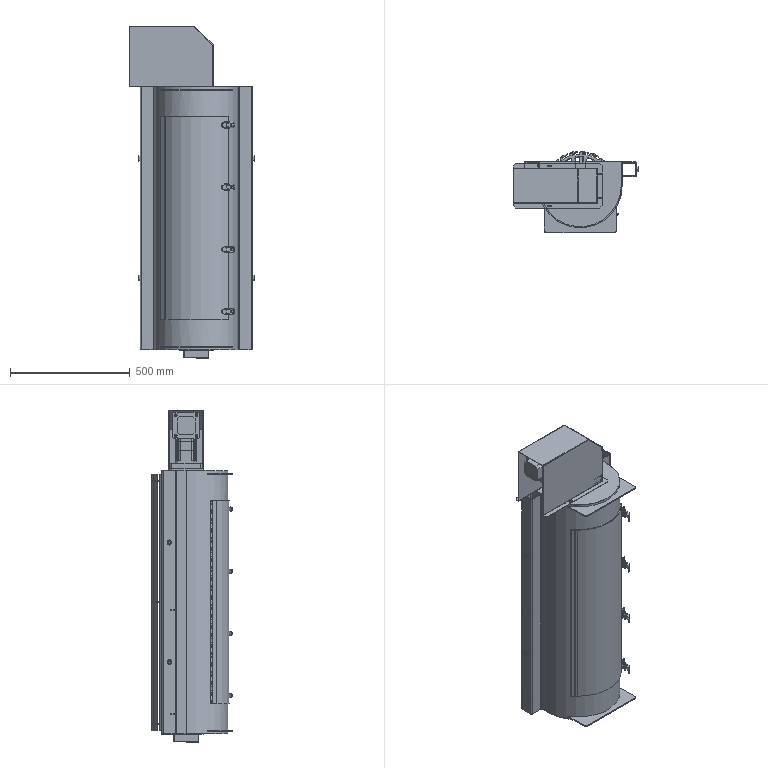Part | SolidWorks | features InContextFeatHolder 8 | 106 solids | 3673 faces | volume 14201492 mm3 | plane 1686 | cylinder 1627 | cone 174 | torus 151 | spline 25 | sphere 10 | commonest cylinder face diameters 10 x210 6.5 x145 4 x104 3.5 x88 4.2 x84 22 x77